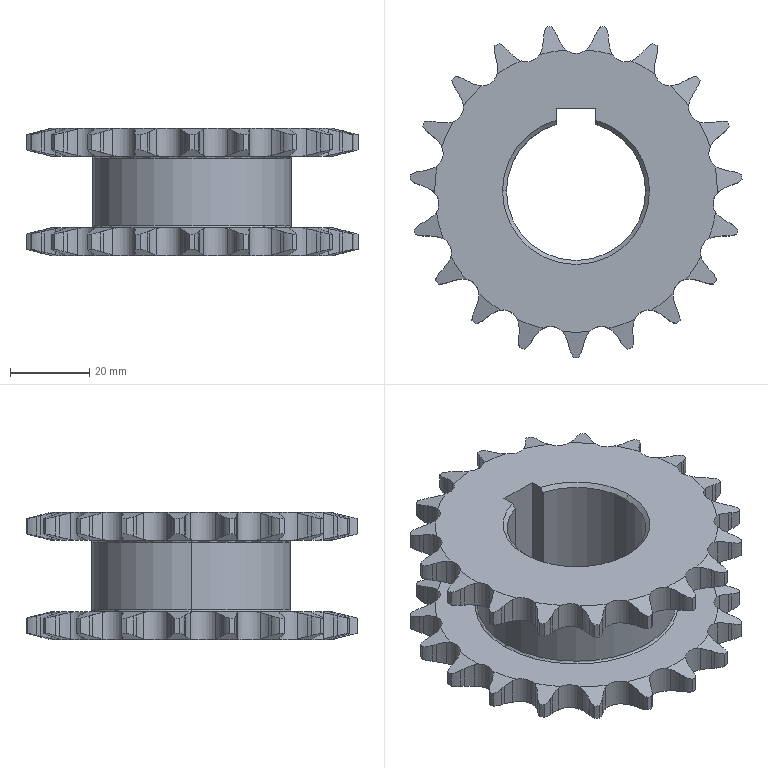Part | STEP file | 02-Small sprocket 3 | 1 solid | 406 faces | box 83.535 x 83.254 x 31.985 mm | volume 63279 mm3 | cylinder 233 | cone 86 | plane 83 | torus 4 | commonest cylinder face diameters 13.162 x76 20.647 x76 7.967 x38 83.727 x38 35 x3 50 x2